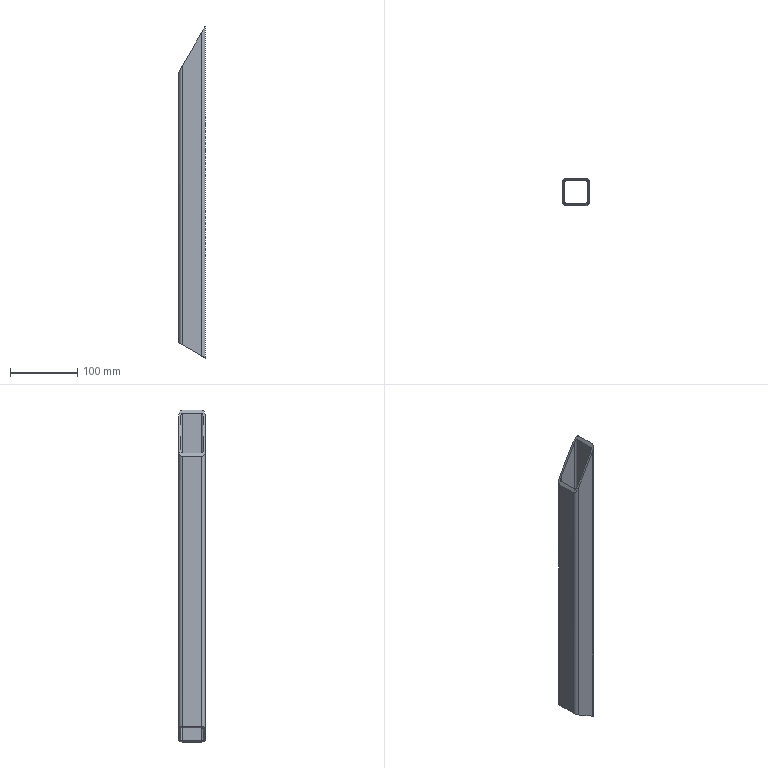Part | STEP file | DIN 59 410 - 40x40x2.9-400 | 1 solid | 20 faces | box 40 x 40 x 495.189 mm | volume 183493 mm3 | plane 10 | cylinder 8 | spline 2 | commonest cylinder face diameters 5.8 x4 11.6 x4